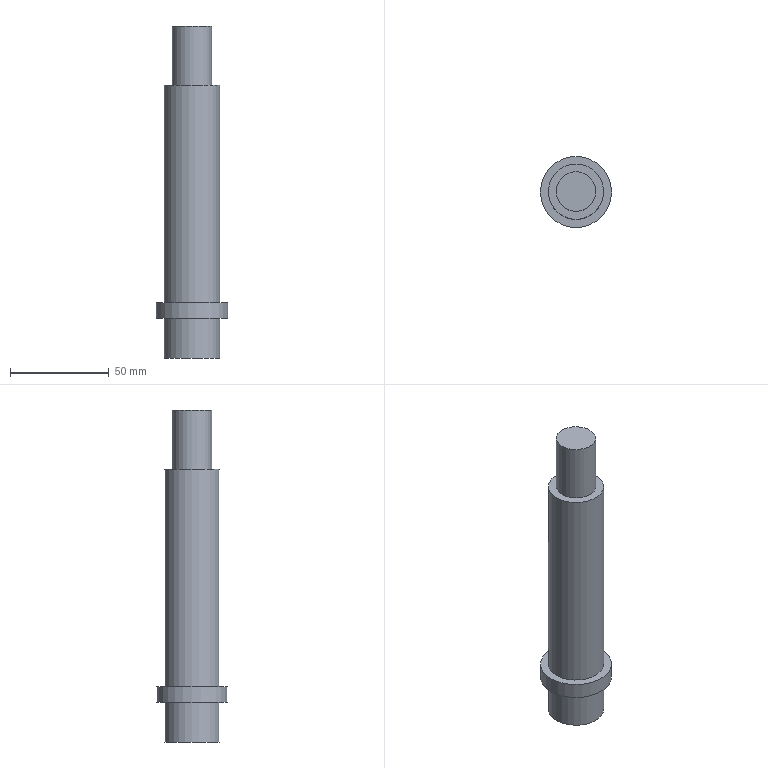Part | NX | features solid 2 | 1 solid | 9 faces | box 36 x 36 x 168 mm | volume 97616 mm3 | plane 5 | cylinder 4 | commonest cylinder face diameters 28 x2 20 x1 36 x1
STEP:
#1=CARTESIAN_POINT('',(16.,-555.,112.));
#2=VERTEX_POINT('',#1);
#3=CARTESIAN_POINT('',(30.,-555.,112.));
#4=DIRECTION('',(0.,0.,-1.));
#5=DIRECTION('',(-1.,0.,0.));
#6=AXIS2_PLACEMENT_3D('',#3,#4,#5);
#7=CIRCLE('',#6,14.);
#8=EDGE_CURVE('',#2,#2,#7,.T.);
#9=ORIENTED_EDGE('',*,*,#8,.T.);
#10=EDGE_LOOP('',(#9));
#11=FACE_BOUND('',#10,.T.);
#12=CARTESIAN_POINT('',(30.,-555.,112.));
#13=DIRECTION('',(0.,0.,-1.));
#14=DIRECTION('',(1.,0.,0.));
#15=AXIS2_PLACEMENT_3D('',#12,#13,#14);
#16=PLANE('',#15);
#17=ADVANCED_FACE('',(#11),#16,.T.);
#18=ORIENTED_EDGE('',*,*,#8,.F.);
#19=EDGE_LOOP('',(#18));
#20=FACE_BOUND('',#19,.T.);
#21=CARTESIAN_POINT('',(44.,-555.,132.));
#22=VERTEX_POINT('',#21);
#23=CARTESIAN_POINT('',(30.,-555.,132.));
#24=DIRECTION('',(0.,0.,1.));
#25=DIRECTION('',(1.,0.,0.));
#26=AXIS2_PLACEMENT_3D('',#23,#24,#25);
#27=CIRCLE('',#26,14.);
#28=EDGE_CURVE('',#22,#22,#27,.F.);
#29=ORIENTED_EDGE('',*,*,#28,.T.);
#30=EDGE_LOOP('',(#29));
#31=FACE_BOUND('',#30,.T.);
#32=CARTESIAN_POINT('',(30.,-555.,332.));
#33=DIRECTION('',(0.,0.,-1.));
#34=DIRECTION('',(1.,0.,0.));
#35=AXIS2_PLACEMENT_3D('',#32,#33,#34);
#36=CYLINDRICAL_SURFACE('',#35,14.);
#37=ADVANCED_FACE('',(#20,#31),#36,.T.);
#38=ORIENTED_EDGE('',*,*,#28,.F.);
#39=EDGE_LOOP('',(#38));
#40=FACE_BOUND('',#39,.T.);
#41=CARTESIAN_POINT('',(12.,-555.,132.));
#42=VERTEX_POINT('',#41);
#43=CARTESIAN_POINT('',(30.,-555.,132.));
#44=DIRECTION('',(0.,0.,-1.));
#45=DIRECTION('',(-1.,0.,0.));
#46=AXIS2_PLACEMENT_3D('',#43,#44,#45);
#47=CIRCLE('',#46,18.);
#48=EDGE_CURVE('',#42,#42,#47,.T.);
#49=ORIENTED_EDGE('',*,*,#48,.T.);
#50=EDGE_LOOP('',(#49));
#51=FACE_BOUND('',#50,.T.);
#52=CARTESIAN_POINT('',(30.,-555.,132.));
#53=DIRECTION('',(0.,0.,-1.));
#54=DIRECTION('',(1.,0.,0.));
#55=AXIS2_PLACEMENT_3D('',#52,#53,#54);
#56=PLANE('',#55);
#57=ADVANCED_FACE('',(#40,#51),#56,.T.);
#58=CARTESIAN_POINT('',(16.,-555.,140.));
#59=VERTEX_POINT('',#58);
#60=CARTESIAN_POINT('',(30.,-555.,140.));
#61=DIRECTION('',(0.,0.,-1.));
#62=DIRECTION('',(-1.,0.,0.));
#63=AXIS2_PLACEMENT_3D('',#60,#61,#62);
#64=CIRCLE('',#63,14.);
#65=EDGE_CURVE('',#59,#59,#64,.T.);
#66=ORIENTED_EDGE('',*,*,#65,.T.);
#67=EDGE_LOOP('',(#66));
#68=FACE_BOUND('',#67,.T.);
#69=CARTESIAN_POINT('',(48.,-555.,140.));
#70=VERTEX_POINT('',#69);
#71=CARTESIAN_POINT('',(30.,-555.,140.));
#72=DIRECTION('',(0.,0.,1.));
#73=DIRECTION('',(1.,0.,0.));
#74=AXIS2_PLACEMENT_3D('',#71,#72,#73);
#75=CIRCLE('',#74,18.);
#76=EDGE_CURVE('',#70,#70,#75,.T.);
#77=ORIENTED_EDGE('',*,*,#76,.T.);
#78=EDGE_LOOP('',(#77));
#79=FACE_BOUND('',#78,.T.);
#80=CARTESIAN_POINT('',(30.,-555.,140.));
#81=DIRECTION('',(0.,0.,1.));
#82=DIRECTION('',(-1.,0.,0.));
#83=AXIS2_PLACEMENT_3D('',#80,#81,#82);
#84=PLANE('',#83);
#85=ADVANCED_FACE('',(#68,#79),#84,.T.);
#86=ORIENTED_EDGE('',*,*,#48,.F.);
#87=EDGE_LOOP('',(#86));
#88=FACE_BOUND('',#87,.T.);
#89=ORIENTED_EDGE('',*,*,#76,.F.);
#90=EDGE_LOOP('',(#89));
#91=FACE_BOUND('',#90,.T.);
#92=CARTESIAN_POINT('',(30.,-555.,340.));
#93=DIRECTION('',(0.,0.,-1.));
#94=DIRECTION('',(1.,0.,0.));
#95=AXIS2_PLACEMENT_3D('',#92,#93,#94);
#96=CYLINDRICAL_SURFACE('',#95,18.);
#97=ADVANCED_FACE('',(#88,#91),#96,.T.);
#98=CARTESIAN_POINT('',(20.,-555.,250.));
#99=VERTEX_POINT('',#98);
#100=CARTESIAN_POINT('',(30.,-555.,250.));
#101=DIRECTION('',(0.,0.,-1.));
#102=DIRECTION('',(-1.,0.,0.));
#103=AXIS2_PLACEMENT_3D('',#100,#101,#102);
#104=CIRCLE('',#103,10.);
#105=EDGE_CURVE('',#99,#99,#104,.T.);
#106=ORIENTED_EDGE('',*,*,#105,.T.);
#107=EDGE_LOOP('',(#106));
#108=FACE_BOUND('',#107,.T.);
#109=CARTESIAN_POINT('',(44.,-555.,250.));
#110=VERTEX_POINT('',#109);
#111=CARTESIAN_POINT('',(30.,-555.,250.));
#112=DIRECTION('',(0.,0.,-1.));
#113=DIRECTION('',(1.,0.,0.));
#114=AXIS2_PLACEMENT_3D('',#111,#112,#113);
#115=CIRCLE('',#114,14.);
#116=EDGE_CURVE('',#110,#110,#115,.F.);
#117=ORIENTED_EDGE('',*,*,#116,.T.);
#118=EDGE_LOOP('',(#117));
#119=FACE_BOUND('',#118,.T.);
#120=CARTESIAN_POINT('',(30.,-555.,250.));
#121=DIRECTION('',(0.,0.,1.));
#122=DIRECTION('',(-1.,0.,0.));
#123=AXIS2_PLACEMENT_3D('',#120,#121,#122);
#124=PLANE('',#123);
#125=ADVANCED_FACE('',(#108,#119),#124,.T.);
#126=ORIENTED_EDGE('',*,*,#65,.F.);
#127=EDGE_LOOP('',(#126));
#128=FACE_BOUND('',#127,.T.);
#129=ORIENTED_EDGE('',*,*,#116,.F.);
#130=EDGE_LOOP('',(#129));
#131=FACE_BOUND('',#130,.T.);
#132=CARTESIAN_POINT('',(30.,-555.,430.));
#133=DIRECTION('',(0.,0.,-1.));
#134=DIRECTION('',(1.,0.,0.));
#135=AXIS2_PLACEMENT_3D('',#132,#133,#134);
#136=CYLINDRICAL_SURFACE('',#135,14.);
#137=ADVANCED_FACE('',(#128,#131),#136,.T.);
#138=CARTESIAN_POINT('',(40.,-555.,280.));
#139=VERTEX_POINT('',#138);
#140=CARTESIAN_POINT('',(30.,-555.,280.));
#141=DIRECTION('',(0.,0.,1.));
#142=DIRECTION('',(1.,0.,0.));
#143=AXIS2_PLACEMENT_3D('',#140,#141,#142);
#144=CIRCLE('',#143,10.);
#145=EDGE_CURVE('',#139,#139,#144,.T.);
#146=ORIENTED_EDGE('',*,*,#145,.T.);
#147=EDGE_LOOP('',(#146));
#148=FACE_BOUND('',#147,.T.);
#149=CARTESIAN_POINT('',(30.,-555.,280.));
#150=DIRECTION('',(0.,0.,1.));
#151=DIRECTION('',(-1.,0.,0.));
#152=AXIS2_PLACEMENT_3D('',#149,#150,#151);
#153=PLANE('',#152);
#154=ADVANCED_FACE('',(#148),#153,.T.);
#155=ORIENTED_EDGE('',*,*,#105,.F.);
#156=EDGE_LOOP('',(#155));
#157=FACE_BOUND('',#156,.T.);
#158=ORIENTED_EDGE('',*,*,#145,.F.);
#159=EDGE_LOOP('',(#158));
#160=FACE_BOUND('',#159,.T.);
#161=CARTESIAN_POINT('',(30.,-555.,280.));
#162=DIRECTION('',(0.,0.,-1.));
#163=DIRECTION('',(1.,0.,0.));
#164=AXIS2_PLACEMENT_3D('',#161,#162,#163);
#165=CYLINDRICAL_SURFACE('',#164,10.);
#166=ADVANCED_FACE('',(#157,#160),#165,.T.);
#167=CLOSED_SHELL('',(#17,#37,#57,#85,#97,#125,#137,#154,#166));
#168=MANIFOLD_SOLID_BREP('',#167);
#169=(LENGTH_UNIT()NAMED_UNIT(*)SI_UNIT(.MILLI.,.METRE.));
#170=UNCERTAINTY_MEASURE_WITH_UNIT(LENGTH_MEASURE(0.00001),#169,'','');
#171=(NAMED_UNIT(*)PLANE_ANGLE_UNIT()SI_UNIT($,.RADIAN.));
#172=(NAMED_UNIT(*)SI_UNIT($,.STERADIAN.)SOLID_ANGLE_UNIT());
#173=(GEOMETRIC_REPRESENTATION_CONTEXT(3)GLOBAL_UNCERTAINTY_ASSIGNED_CONTEXT((#170))GLOBAL_UNIT_ASSIGNED_CONTEXT((#169,#171,#172))REPRESENTATION_CONTEXT('',''));
#174=ADVANCED_BREP_SHAPE_REPRESENTATION('',(#168),#173);